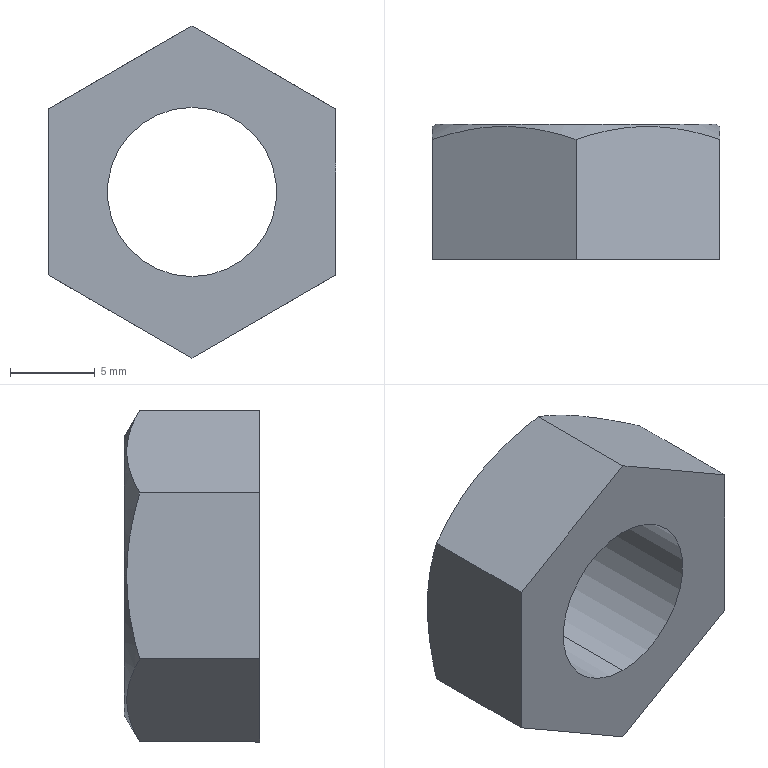Part | STEP file | NN42-M10 | 1 solid | 12 faces | box 17 x 8 x 19.63 mm | volume 1364 mm3 | plane 8 | cylinder 2 | cone 2 | commonest cylinder face diameters 10 x2
STEP:
#1=CARTESIAN_POINT('',(0.,8.,5.));
#2=VERTEX_POINT('',#1);
#3=CARTESIAN_POINT('',(0.,8.,-5.));
#4=VERTEX_POINT('',#3);
#5=CARTESIAN_POINT('',(0.,8.,0.));
#6=DIRECTION('',(0.,-1.,0.));
#7=DIRECTION('',(0.,0.,-1.));
#8=AXIS2_PLACEMENT_3D('',#5,#6,#7);
#9=CIRCLE('',#8,5.);
#10=EDGE_CURVE('',#2,#4,#9,.T.);
#11=ORIENTED_EDGE('',*,*,#10,.F.);
#12=CARTESIAN_POINT('',(0.,0.,5.));
#13=VERTEX_POINT('',#12);
#14=CARTESIAN_POINT('',(0.,8.,5.));
#15=DIRECTION('',(0.,-1.,0.));
#16=VECTOR('',#15,1000.);
#17=LINE('',#14,#16);
#18=EDGE_CURVE('',#2,#13,#17,.T.);
#19=ORIENTED_EDGE('',*,*,#18,.T.);
#20=CARTESIAN_POINT('',(0.,0.,-5.));
#21=VERTEX_POINT('',#20);
#22=CARTESIAN_POINT('',(0.,0.,0.));
#23=DIRECTION('',(0.,1.,0.));
#24=DIRECTION('',(0.,0.,1.));
#25=AXIS2_PLACEMENT_3D('',#22,#23,#24);
#26=CIRCLE('',#25,5.);
#27=EDGE_CURVE('',#21,#13,#26,.T.);
#28=ORIENTED_EDGE('',*,*,#27,.F.);
#29=CARTESIAN_POINT('',(0.,8.,-5.));
#30=DIRECTION('',(0.,-1.,0.));
#31=VECTOR('',#30,1000.);
#32=LINE('',#29,#31);
#33=EDGE_CURVE('',#4,#21,#32,.T.);
#34=ORIENTED_EDGE('',*,*,#33,.F.);
#35=EDGE_LOOP('',(#11,#19,#28,#34));
#36=FACE_OUTER_BOUND('',#35,.T.);
#37=CARTESIAN_POINT('',(0.,8.,0.));
#38=DIRECTION('',(0.,-1.,0.));
#39=DIRECTION('',(0.,0.,-1.));
#40=AXIS2_PLACEMENT_3D('',#37,#38,#39);
#41=CYLINDRICAL_SURFACE('',#40,5.);
#42=ADVANCED_FACE('',(#36),#41,.F.);
#43=CARTESIAN_POINT('',(8.25,8.,0.));
#44=VERTEX_POINT('',#43);
#45=CARTESIAN_POINT('',(-8.25,8.,0.));
#46=VERTEX_POINT('',#45);
#47=CARTESIAN_POINT('',(0.,8.,0.));
#48=DIRECTION('',(0.,-1.,0.));
#49=DIRECTION('',(1.,0.,0.));
#50=AXIS2_PLACEMENT_3D('',#47,#48,#49);
#51=CIRCLE('',#50,8.25);
#52=EDGE_CURVE('',#44,#46,#51,.T.);
#53=ORIENTED_EDGE('',*,*,#52,.T.);
#54=CARTESIAN_POINT('',(-8.5,7.856,0.));
#55=VERTEX_POINT('',#54);
#56=CARTESIAN_POINT('',(-8.25,8.,0.));
#57=DIRECTION('',(-0.866,-0.5,0.));
#58=VECTOR('',#57,1000.);
#59=LINE('',#56,#58);
#60=EDGE_CURVE('',#46,#55,#59,.T.);
#61=ORIENTED_EDGE('',*,*,#60,.T.);
#62=CARTESIAN_POINT('',(-8.5,7.096,4.907));
#63=VERTEX_POINT('',#62);
#64=CARTESIAN_POINT('',(-8.5,7.096,4.907));
#65=CARTESIAN_POINT('',(-8.5,7.327,4.108));
#66=CARTESIAN_POINT('',(-8.5,7.518,3.302));
#67=CARTESIAN_POINT('',(-8.5,7.783,1.668));
#68=CARTESIAN_POINT('',(-8.5,7.856,0.8404));
#69=CARTESIAN_POINT('',(-8.5,7.856,0.));
#70=B_SPLINE_CURVE_WITH_KNOTS('',3,(#64,#65,#66,#67,#68,#69),.UNSPECIFIED.,.F.,.F.,(4,2,4),(0.01071,0.0132,0.0157),.UNSPECIFIED.);
#71=EDGE_CURVE('',#63,#55,#70,.T.);
#72=ORIENTED_EDGE('',*,*,#71,.F.);
#73=CARTESIAN_POINT('',(0.,7.096,9.815));
#74=VERTEX_POINT('',#73);
#75=CARTESIAN_POINT('',(0.,7.096,9.815));
#76=CARTESIAN_POINT('',(-0.6939,7.328,9.414));
#77=CARTESIAN_POINT('',(-1.393,7.518,9.011));
#78=CARTESIAN_POINT('',(-2.806,7.783,8.195));
#79=CARTESIAN_POINT('',(-3.519,7.855,7.783));
#80=CARTESIAN_POINT('',(-4.603,7.856,7.157));
#81=CARTESIAN_POINT('',(-4.966,7.838,6.948));
#82=CARTESIAN_POINT('',(-5.684,7.769,6.533));
#83=CARTESIAN_POINT('',(-6.041,7.718,6.327));
#84=CARTESIAN_POINT('',(-7.105,7.519,5.713));
#85=CARTESIAN_POINT('',(-7.805,7.328,5.309));
#86=CARTESIAN_POINT('',(-8.5,7.096,4.907));
#87=B_SPLINE_CURVE_WITH_KNOTS('',3,(#75,#76,#77,#78,#79,#80,#81,#82,#83,#84,#85,#86),.UNSPECIFIED.,.F.,.F.,(4,2,2,2,2,4),(0.000000238,0.002478,0.004957,0.006196,0.007435,0.009913),.UNSPECIFIED.);
#88=EDGE_CURVE('',#74,#63,#87,.T.);
#89=ORIENTED_EDGE('',*,*,#88,.F.);
#90=CARTESIAN_POINT('',(8.5,7.096,4.907));
#91=VERTEX_POINT('',#90);
#92=CARTESIAN_POINT('',(8.5,7.096,4.907));
#93=CARTESIAN_POINT('',(7.806,7.328,5.308));
#94=CARTESIAN_POINT('',(7.107,7.518,5.712));
#95=CARTESIAN_POINT('',(5.694,7.783,6.527));
#96=CARTESIAN_POINT('',(4.981,7.855,6.939));
#97=CARTESIAN_POINT('',(3.897,7.856,7.565));
#98=CARTESIAN_POINT('',(3.534,7.838,7.775));
#99=CARTESIAN_POINT('',(2.816,7.769,8.189));
#100=CARTESIAN_POINT('',(2.459,7.718,8.395));
#101=CARTESIAN_POINT('',(1.395,7.519,9.009));
#102=CARTESIAN_POINT('',(0.6948,7.328,9.414));
#103=CARTESIAN_POINT('',(0.,7.096,9.815));
#104=B_SPLINE_CURVE_WITH_KNOTS('',3,(#92,#93,#94,#95,#96,#97,#98,#99,#100,#101,#102,#103),.UNSPECIFIED.,.F.,.F.,(4,2,2,2,2,4),(0.000000238,0.002478,0.004957,0.006196,0.007435,0.009913),.UNSPECIFIED.);
#105=EDGE_CURVE('',#91,#74,#104,.T.);
#106=ORIENTED_EDGE('',*,*,#105,.F.);
#107=CARTESIAN_POINT('',(8.5,7.856,0.));
#108=VERTEX_POINT('',#107);
#109=CARTESIAN_POINT('',(8.5,7.856,0.));
#110=CARTESIAN_POINT('',(8.5,7.856,0.8399));
#111=CARTESIAN_POINT('',(8.5,7.782,1.669));
#112=CARTESIAN_POINT('',(8.5,7.518,3.303));
#113=CARTESIAN_POINT('',(8.5,7.327,4.109));
#114=CARTESIAN_POINT('',(8.5,7.096,4.907));
#115=B_SPLINE_CURVE_WITH_KNOTS('',3,(#109,#110,#111,#112,#113,#114),.UNSPECIFIED.,.F.,.F.,(4,2,4),(0.0157,0.01819,0.02069),.UNSPECIFIED.);
#116=EDGE_CURVE('',#108,#91,#115,.T.);
#117=ORIENTED_EDGE('',*,*,#116,.F.);
#118=CARTESIAN_POINT('',(8.25,8.,0.));
#119=DIRECTION('',(0.866,-0.5,0.));
#120=VECTOR('',#119,1000.);
#121=LINE('',#118,#120);
#122=EDGE_CURVE('',#44,#108,#121,.T.);
#123=ORIENTED_EDGE('',*,*,#122,.F.);
#124=EDGE_LOOP('',(#53,#61,#72,#89,#106,#117,#123));
#125=FACE_OUTER_BOUND('',#124,.T.);
#126=CARTESIAN_POINT('',(0.,8.,0.));
#127=DIRECTION('',(0.,-1.,0.));
#128=DIRECTION('',(1.,0.,0.));
#129=AXIS2_PLACEMENT_3D('',#126,#127,#128);
#130=CONICAL_SURFACE('',#129,8.25,1.047);
#131=ADVANCED_FACE('',(#125),#130,.T.);
#132=ORIENTED_EDGE('',*,*,#60,.F.);
#133=CARTESIAN_POINT('',(0.,8.,0.));
#134=DIRECTION('',(0.,-1.,0.));
#135=DIRECTION('',(1.,0.,0.));
#136=AXIS2_PLACEMENT_3D('',#133,#134,#135);
#137=CIRCLE('',#136,8.25);
#138=EDGE_CURVE('',#46,#44,#137,.T.);
#139=ORIENTED_EDGE('',*,*,#138,.T.);
#140=ORIENTED_EDGE('',*,*,#122,.T.);
#141=CARTESIAN_POINT('',(8.5,7.096,-4.907));
#142=VERTEX_POINT('',#141);
#143=CARTESIAN_POINT('',(8.5,7.096,-4.907));
#144=CARTESIAN_POINT('',(8.5,7.327,-4.108));
#145=CARTESIAN_POINT('',(8.5,7.518,-3.302));
#146=CARTESIAN_POINT('',(8.5,7.783,-1.668));
#147=CARTESIAN_POINT('',(8.5,7.856,-0.8404));
#148=CARTESIAN_POINT('',(8.5,7.856,0.));
#149=B_SPLINE_CURVE_WITH_KNOTS('',3,(#143,#144,#145,#146,#147,#148),.UNSPECIFIED.,.F.,.F.,(4,2,4),(0.01071,0.0132,0.0157),.UNSPECIFIED.);
#150=EDGE_CURVE('',#142,#108,#149,.T.);
#151=ORIENTED_EDGE('',*,*,#150,.F.);
#152=CARTESIAN_POINT('',(0.,7.096,-9.815));
#153=VERTEX_POINT('',#152);
#154=CARTESIAN_POINT('',(0.,7.096,-9.815));
#155=CARTESIAN_POINT('',(0.6939,7.328,-9.414));
#156=CARTESIAN_POINT('',(1.393,7.518,-9.011));
#157=CARTESIAN_POINT('',(2.806,7.783,-8.195));
#158=CARTESIAN_POINT('',(3.519,7.855,-7.783));
#159=CARTESIAN_POINT('',(4.603,7.856,-7.157));
#160=CARTESIAN_POINT('',(4.966,7.838,-6.948));
#161=CARTESIAN_POINT('',(5.684,7.769,-6.533));
#162=CARTESIAN_POINT('',(6.041,7.718,-6.327));
#163=CARTESIAN_POINT('',(7.105,7.519,-5.713));
#164=CARTESIAN_POINT('',(7.805,7.328,-5.309));
#165=CARTESIAN_POINT('',(8.5,7.096,-4.907));
#166=B_SPLINE_CURVE_WITH_KNOTS('',3,(#154,#155,#156,#157,#158,#159,#160,#161,#162,#163,#164,#165),.UNSPECIFIED.,.F.,.F.,(4,2,2,2,2,4),(0.000000238,0.002478,0.004957,0.006196,0.007435,0.009913),.UNSPECIFIED.);
#167=EDGE_CURVE('',#153,#142,#166,.T.);
#168=ORIENTED_EDGE('',*,*,#167,.F.);
#169=CARTESIAN_POINT('',(-8.5,7.096,-4.907));
#170=VERTEX_POINT('',#169);
#171=CARTESIAN_POINT('',(-8.5,7.096,-4.907));
#172=CARTESIAN_POINT('',(-7.806,7.328,-5.308));
#173=CARTESIAN_POINT('',(-7.107,7.518,-5.712));
#174=CARTESIAN_POINT('',(-5.694,7.783,-6.527));
#175=CARTESIAN_POINT('',(-4.981,7.855,-6.939));
#176=CARTESIAN_POINT('',(-3.897,7.856,-7.565));
#177=CARTESIAN_POINT('',(-3.534,7.838,-7.775));
#178=CARTESIAN_POINT('',(-2.816,7.769,-8.189));
#179=CARTESIAN_POINT('',(-2.459,7.718,-8.395));
#180=CARTESIAN_POINT('',(-1.395,7.519,-9.009));
#181=CARTESIAN_POINT('',(-0.6948,7.328,-9.414));
#182=CARTESIAN_POINT('',(0.,7.096,-9.815));
#183=B_SPLINE_CURVE_WITH_KNOTS('',3,(#171,#172,#173,#174,#175,#176,#177,#178,#179,#180,#181,#182),.UNSPECIFIED.,.F.,.F.,(4,2,2,2,2,4),(0.000000238,0.002478,0.004957,0.006196,0.007435,0.009913),.UNSPECIFIED.);
#184=EDGE_CURVE('',#170,#153,#183,.T.);
#185=ORIENTED_EDGE('',*,*,#184,.F.);
#186=CARTESIAN_POINT('',(-8.5,7.856,0.));
#187=CARTESIAN_POINT('',(-8.5,7.856,-0.8399));
#188=CARTESIAN_POINT('',(-8.5,7.782,-1.669));
#189=CARTESIAN_POINT('',(-8.5,7.518,-3.303));
#190=CARTESIAN_POINT('',(-8.5,7.327,-4.109));
#191=CARTESIAN_POINT('',(-8.5,7.096,-4.907));
#192=B_SPLINE_CURVE_WITH_KNOTS('',3,(#186,#187,#188,#189,#190,#191),.UNSPECIFIED.,.F.,.F.,(4,2,4),(0.0157,0.01819,0.02069),.UNSPECIFIED.);
#193=EDGE_CURVE('',#55,#170,#192,.T.);
#194=ORIENTED_EDGE('',*,*,#193,.F.);
#195=EDGE_LOOP('',(#132,#139,#140,#151,#168,#185,#194));
#196=FACE_OUTER_BOUND('',#195,.T.);
#197=CARTESIAN_POINT('',(0.,8.,0.));
#198=DIRECTION('',(0.,-1.,0.));
#199=DIRECTION('',(1.,0.,0.));
#200=AXIS2_PLACEMENT_3D('',#197,#198,#199);
#201=CONICAL_SURFACE('',#200,8.25,1.047);
#202=ADVANCED_FACE('',(#196),#201,.T.);
#203=CARTESIAN_POINT('',(0.,8.,0.));
#204=DIRECTION('',(0.,-1.,0.));
#205=DIRECTION('',(0.,0.,-1.));
#206=AXIS2_PLACEMENT_3D('',#203,#204,#205);
#207=CIRCLE('',#206,5.);
#208=EDGE_CURVE('',#4,#2,#207,.T.);
#209=ORIENTED_EDGE('',*,*,#208,.T.);
#210=ORIENTED_EDGE('',*,*,#10,.T.);
#211=EDGE_LOOP('',(#209,#210));
#212=FACE_BOUND('',#211,.T.);
#213=ORIENTED_EDGE('',*,*,#52,.F.);
#214=ORIENTED_EDGE('',*,*,#138,.F.);
#215=EDGE_LOOP('',(#213,#214));
#216=FACE_OUTER_BOUND('',#215,.T.);
#217=CARTESIAN_POINT('',(0.,8.,0.));
#218=DIRECTION('',(0.,1.,0.));
#219=DIRECTION('',(-1.,0.,0.));
#220=AXIS2_PLACEMENT_3D('',#217,#218,#219);
#221=PLANE('',#220);
#222=ADVANCED_FACE('',(#212,#216),#221,.T.);
#223=ORIENTED_EDGE('',*,*,#150,.T.);
#224=ORIENTED_EDGE('',*,*,#116,.T.);
#225=CARTESIAN_POINT('',(8.5,0.,4.907));
#226=VERTEX_POINT('',#225);
#227=CARTESIAN_POINT('',(8.5,0.,4.907));
#228=DIRECTION('',(0.,1.,0.));
#229=VECTOR('',#228,1000.);
#230=LINE('',#227,#229);
#231=EDGE_CURVE('',#226,#91,#230,.T.);
#232=ORIENTED_EDGE('',*,*,#231,.F.);
#233=CARTESIAN_POINT('',(8.5,0.,-4.907));
#234=VERTEX_POINT('',#233);
#235=CARTESIAN_POINT('',(8.5,0.,-4.907));
#236=DIRECTION('',(0.,0.,1.));
#237=VECTOR('',#236,1000.);
#238=LINE('',#235,#237);
#239=EDGE_CURVE('',#234,#226,#238,.T.);
#240=ORIENTED_EDGE('',*,*,#239,.F.);
#241=CARTESIAN_POINT('',(8.5,0.,-4.907));
#242=DIRECTION('',(0.,1.,0.));
#243=VECTOR('',#242,1000.);
#244=LINE('',#241,#243);
#245=EDGE_CURVE('',#234,#142,#244,.T.);
#246=ORIENTED_EDGE('',*,*,#245,.T.);
#247=EDGE_LOOP('',(#223,#224,#232,#240,#246));
#248=FACE_OUTER_BOUND('',#247,.T.);
#249=CARTESIAN_POINT('',(8.5,7.096,-4.907));
#250=DIRECTION('',(-1.,0.,0.));
#251=DIRECTION('',(0.,0.,-1.));
#252=AXIS2_PLACEMENT_3D('',#249,#250,#251);
#253=PLANE('',#252);
#254=ADVANCED_FACE('',(#248),#253,.F.);
#255=ORIENTED_EDGE('',*,*,#167,.T.);
#256=ORIENTED_EDGE('',*,*,#245,.F.);
#257=CARTESIAN_POINT('',(0.,0.,-9.815));
#258=VERTEX_POINT('',#257);
#259=CARTESIAN_POINT('',(0.,0.,-9.815));
#260=DIRECTION('',(0.866,0.,0.5));
#261=VECTOR('',#260,1000.);
#262=LINE('',#259,#261);
#263=EDGE_CURVE('',#258,#234,#262,.T.);
#264=ORIENTED_EDGE('',*,*,#263,.F.);
#265=CARTESIAN_POINT('',(0.,0.,-9.815));
#266=DIRECTION('',(0.,1.,0.));
#267=VECTOR('',#266,1000.);
#268=LINE('',#265,#267);
#269=EDGE_CURVE('',#258,#153,#268,.T.);
#270=ORIENTED_EDGE('',*,*,#269,.T.);
#271=EDGE_LOOP('',(#255,#256,#264,#270));
#272=FACE_OUTER_BOUND('',#271,.T.);
#273=CARTESIAN_POINT('',(0.,7.096,-9.815));
#274=DIRECTION('',(-0.5,0.,0.866));
#275=DIRECTION('',(-0.866,0.,-0.5));
#276=AXIS2_PLACEMENT_3D('',#273,#274,#275);
#277=PLANE('',#276);
#278=ADVANCED_FACE('',(#272),#277,.F.);
#279=ORIENTED_EDGE('',*,*,#184,.T.);
#280=ORIENTED_EDGE('',*,*,#269,.F.);
#281=CARTESIAN_POINT('',(-8.5,0.,-4.907));
#282=VERTEX_POINT('',#281);
#283=CARTESIAN_POINT('',(-8.5,0.,-4.907));
#284=DIRECTION('',(0.866,0.,-0.5));
#285=VECTOR('',#284,1000.);
#286=LINE('',#283,#285);
#287=EDGE_CURVE('',#282,#258,#286,.T.);
#288=ORIENTED_EDGE('',*,*,#287,.F.);
#289=CARTESIAN_POINT('',(-8.5,0.,-4.907));
#290=DIRECTION('',(0.,1.,0.));
#291=VECTOR('',#290,1000.);
#292=LINE('',#289,#291);
#293=EDGE_CURVE('',#282,#170,#292,.T.);
#294=ORIENTED_EDGE('',*,*,#293,.T.);
#295=EDGE_LOOP('',(#279,#280,#288,#294));
#296=FACE_OUTER_BOUND('',#295,.T.);
#297=CARTESIAN_POINT('',(-8.5,7.096,-4.907));
#298=DIRECTION('',(0.5,0.,0.866));
#299=DIRECTION('',(-0.866,0.,0.5));
#300=AXIS2_PLACEMENT_3D('',#297,#298,#299);
#301=PLANE('',#300);
#302=ADVANCED_FACE('',(#296),#301,.F.);
#303=ORIENTED_EDGE('',*,*,#71,.T.);
#304=ORIENTED_EDGE('',*,*,#193,.T.);
#305=ORIENTED_EDGE('',*,*,#293,.F.);
#306=CARTESIAN_POINT('',(-8.5,0.,4.907));
#307=VERTEX_POINT('',#306);
#308=CARTESIAN_POINT('',(-8.5,0.,4.907));
#309=DIRECTION('',(0.,0.,-1.));
#310=VECTOR('',#309,1000.);
#311=LINE('',#308,#310);
#312=EDGE_CURVE('',#307,#282,#311,.T.);
#313=ORIENTED_EDGE('',*,*,#312,.F.);
#314=CARTESIAN_POINT('',(-8.5,0.,4.907));
#315=DIRECTION('',(0.,1.,0.));
#316=VECTOR('',#315,1000.);
#317=LINE('',#314,#316);
#318=EDGE_CURVE('',#307,#63,#317,.T.);
#319=ORIENTED_EDGE('',*,*,#318,.T.);
#320=EDGE_LOOP('',(#303,#304,#305,#313,#319));
#321=FACE_OUTER_BOUND('',#320,.T.);
#322=CARTESIAN_POINT('',(-8.5,7.096,4.907));
#323=DIRECTION('',(1.,0.,0.));
#324=DIRECTION('',(0.,0.,1.));
#325=AXIS2_PLACEMENT_3D('',#322,#323,#324);
#326=PLANE('',#325);
#327=ADVANCED_FACE('',(#321),#326,.F.);
#328=ORIENTED_EDGE('',*,*,#88,.T.);
#329=ORIENTED_EDGE('',*,*,#318,.F.);
#330=CARTESIAN_POINT('',(0.,0.,9.815));
#331=VERTEX_POINT('',#330);
#332=CARTESIAN_POINT('',(0.,0.,9.815));
#333=DIRECTION('',(-0.866,0.,-0.5));
#334=VECTOR('',#333,1000.);
#335=LINE('',#332,#334);
#336=EDGE_CURVE('',#331,#307,#335,.T.);
#337=ORIENTED_EDGE('',*,*,#336,.F.);
#338=CARTESIAN_POINT('',(0.,0.,9.815));
#339=DIRECTION('',(0.,1.,0.));
#340=VECTOR('',#339,1000.);
#341=LINE('',#338,#340);
#342=EDGE_CURVE('',#331,#74,#341,.T.);
#343=ORIENTED_EDGE('',*,*,#342,.T.);
#344=EDGE_LOOP('',(#328,#329,#337,#343));
#345=FACE_OUTER_BOUND('',#344,.T.);
#346=CARTESIAN_POINT('',(0.,7.096,9.815));
#347=DIRECTION('',(0.5,0.,-0.866));
#348=DIRECTION('',(0.866,0.,0.5));
#349=AXIS2_PLACEMENT_3D('',#346,#347,#348);
#350=PLANE('',#349);
#351=ADVANCED_FACE('',(#345),#350,.F.);
#352=ORIENTED_EDGE('',*,*,#105,.T.);
#353=ORIENTED_EDGE('',*,*,#342,.F.);
#354=CARTESIAN_POINT('',(8.5,0.,4.907));
#355=DIRECTION('',(-0.866,0.,0.5));
#356=VECTOR('',#355,1000.);
#357=LINE('',#354,#356);
#358=EDGE_CURVE('',#226,#331,#357,.T.);
#359=ORIENTED_EDGE('',*,*,#358,.F.);
#360=ORIENTED_EDGE('',*,*,#231,.T.);
#361=EDGE_LOOP('',(#352,#353,#359,#360));
#362=FACE_OUTER_BOUND('',#361,.T.);
#363=CARTESIAN_POINT('',(8.5,7.096,4.907));
#364=DIRECTION('',(-0.5,0.,-0.866));
#365=DIRECTION('',(0.866,0.,-0.5));
#366=AXIS2_PLACEMENT_3D('',#363,#364,#365);
#367=PLANE('',#366);
#368=ADVANCED_FACE('',(#362),#367,.F.);
#369=ORIENTED_EDGE('',*,*,#27,.T.);
#370=CARTESIAN_POINT('',(0.,0.,0.));
#371=DIRECTION('',(0.,1.,0.));
#372=DIRECTION('',(0.,0.,1.));
#373=AXIS2_PLACEMENT_3D('',#370,#371,#372);
#374=CIRCLE('',#373,5.);
#375=EDGE_CURVE('',#13,#21,#374,.T.);
#376=ORIENTED_EDGE('',*,*,#375,.T.);
#377=EDGE_LOOP('',(#369,#376));
#378=FACE_BOUND('',#377,.T.);
#379=ORIENTED_EDGE('',*,*,#358,.T.);
#380=ORIENTED_EDGE('',*,*,#336,.T.);
#381=ORIENTED_EDGE('',*,*,#312,.T.);
#382=ORIENTED_EDGE('',*,*,#287,.T.);
#383=ORIENTED_EDGE('',*,*,#263,.T.);
#384=ORIENTED_EDGE('',*,*,#239,.T.);
#385=EDGE_LOOP('',(#379,#380,#381,#382,#383,#384));
#386=FACE_OUTER_BOUND('',#385,.T.);
#387=CARTESIAN_POINT('',(0.,0.,0.));
#388=DIRECTION('',(0.,-1.,0.));
#389=DIRECTION('',(0.,0.,1.));
#390=AXIS2_PLACEMENT_3D('',#387,#388,#389);
#391=PLANE('',#390);
#392=ADVANCED_FACE('',(#378,#386),#391,.T.);
#393=ORIENTED_EDGE('',*,*,#18,.F.);
#394=ORIENTED_EDGE('',*,*,#208,.F.);
#395=ORIENTED_EDGE('',*,*,#33,.T.);
#396=ORIENTED_EDGE('',*,*,#375,.F.);
#397=EDGE_LOOP('',(#393,#394,#395,#396));
#398=FACE_OUTER_BOUND('',#397,.T.);
#399=CARTESIAN_POINT('',(0.,8.,0.));
#400=DIRECTION('',(0.,-1.,0.));
#401=DIRECTION('',(0.,0.,-1.));
#402=AXIS2_PLACEMENT_3D('',#399,#400,#401);
#403=CYLINDRICAL_SURFACE('',#402,5.);
#404=ADVANCED_FACE('',(#398),#403,.F.);
#405=CLOSED_SHELL('',(#42,#131,#202,#222,#254,#278,#302,#327,#351,#368,#392,#404));
#406=MANIFOLD_SOLID_BREP('',#405);
#407=CARTESIAN_POINT('',(0.,0.,0.));
#408=DIRECTION('',(0.,0.,1.));
#409=DIRECTION('',(1.,0.,0.));
#410=AXIS2_PLACEMENT_3D('',#407,#408,#409);
#411=(LENGTH_UNIT()NAMED_UNIT(*)SI_UNIT(.MILLI.,.METRE.));
#412=UNCERTAINTY_MEASURE_WITH_UNIT(LENGTH_MEASURE(0.00001),#411,'','');
#413=(NAMED_UNIT(*)PLANE_ANGLE_UNIT()SI_UNIT($,.RADIAN.));
#414=(NAMED_UNIT(*)SI_UNIT($,.STERADIAN.)SOLID_ANGLE_UNIT());
#415=(GEOMETRIC_REPRESENTATION_CONTEXT(3)GLOBAL_UNCERTAINTY_ASSIGNED_CONTEXT((#412))GLOBAL_UNIT_ASSIGNED_CONTEXT((#411,#413,#414))REPRESENTATION_CONTEXT('',''));
#416=ADVANCED_BREP_SHAPE_REPRESENTATION('',(#406,#410),#415);